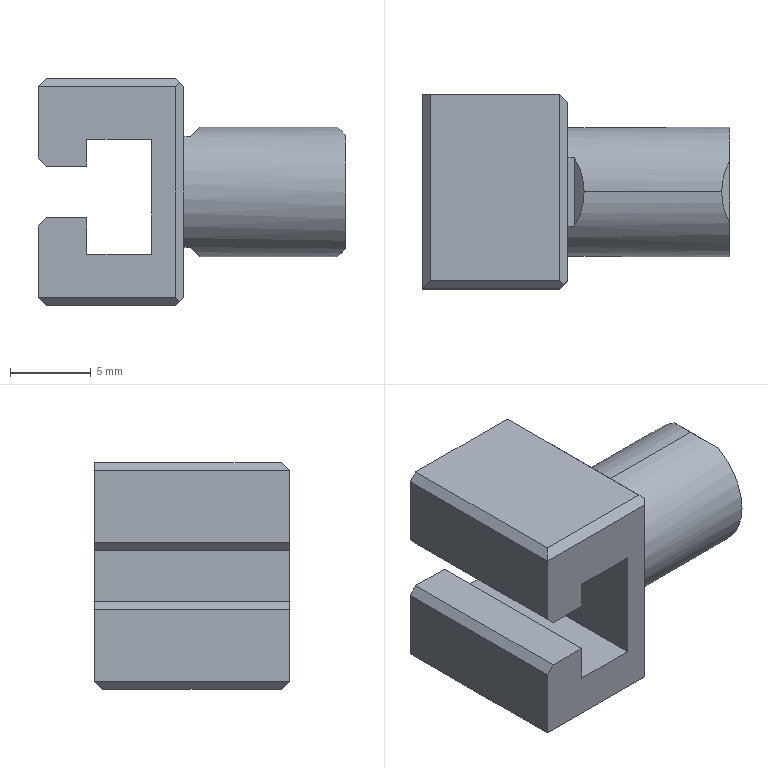Part | STEP file | detection union | 1 solid | 34 faces | box 19 x 12 x 14 mm | volume 1541 mm3 | plane 32 | cylinder 2 | commonest cylinder face diameters 8 x2